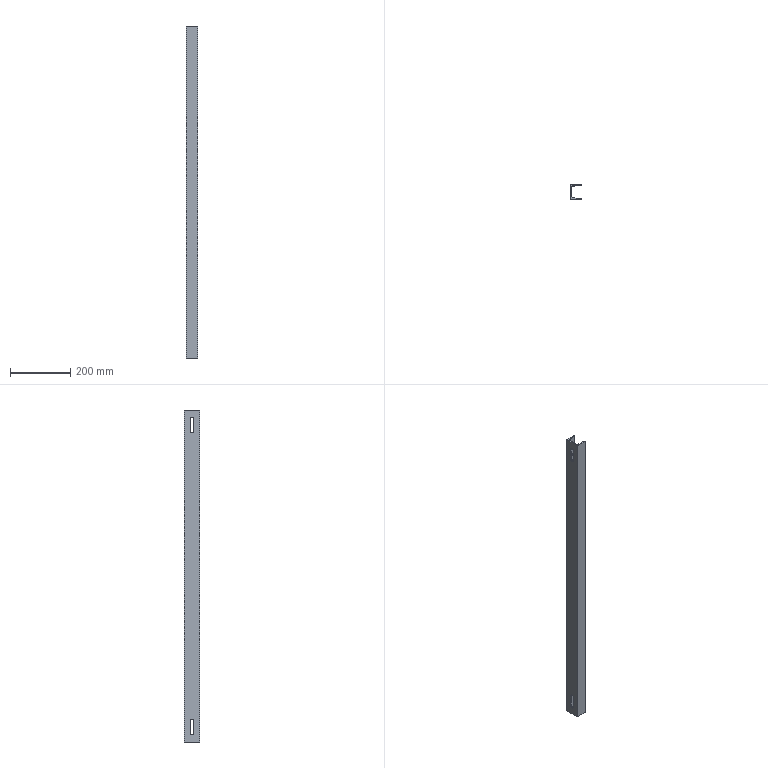Part | SolidWorks | features BaseBody 1 | 1 solid | 30 faces | box 37 x 50 x 1100 mm | volume 540936 mm3 | cylinder 18 | plane 12 | commonest cylinder face diameters 7 x6 12 x6 10.5 x4 14 x2
STEP:
#1=CARTESIAN_POINT('',(20.,21.002,446.5));
#2=VERTEX_POINT('',#1);
#3=CARTESIAN_POINT('',(20.,25.,446.5));
#4=VERTEX_POINT('',#3);
#5=CARTESIAN_POINT('',(20.,15.,446.5));
#6=DIRECTION('',(0.,1.,0.));
#7=VECTOR('',#6,1000.);
#8=LINE('',#5,#7);
#9=EDGE_CURVE('',#2,#4,#8,.T.);
#10=ORIENTED_EDGE('',*,*,#9,.F.);
#11=CARTESIAN_POINT('',(20.,21.002,453.5));
#12=VERTEX_POINT('',#11);
#13=CARTESIAN_POINT('',(20.,21.002,453.5));
#14=CARTESIAN_POINT('',(27.,21.259,453.5));
#15=CARTESIAN_POINT('',(27.,21.259,446.5));
#16=CARTESIAN_POINT('',(20.,21.002,446.5));
#17=(BOUNDED_CURVE()B_SPLINE_CURVE(3,(#13,#14,#15,#16),.UNSPECIFIED.,.F.,.F.)B_SPLINE_CURVE_WITH_KNOTS((4,4),(4.712,7.854),.UNSPECIFIED.)CURVE()GEOMETRIC_REPRESENTATION_ITEM()RATIONAL_B_SPLINE_CURVE((1.,0.3333,0.3333,1.))REPRESENTATION_ITEM(''));
#18=EDGE_CURVE('',#12,#2,#17,.T.);
#19=ORIENTED_EDGE('',*,*,#18,.F.);
#20=CARTESIAN_POINT('',(20.,25.,453.5));
#21=VERTEX_POINT('',#20);
#22=CARTESIAN_POINT('',(20.,15.,453.5));
#23=DIRECTION('',(0.,1.,0.));
#24=VECTOR('',#23,1000.);
#25=LINE('',#22,#24);
#26=EDGE_CURVE('',#12,#21,#25,.T.);
#27=ORIENTED_EDGE('',*,*,#26,.T.);
#28=CARTESIAN_POINT('',(20.,25.,450.));
#29=DIRECTION('',(0.,1.,0.));
#30=DIRECTION('',(0.,0.,1.));
#31=AXIS2_PLACEMENT_3D('',#28,#29,#30);
#32=CIRCLE('',#31,3.5);
#33=EDGE_CURVE('',#21,#4,#32,.T.);
#34=ORIENTED_EDGE('',*,*,#33,.T.);
#35=EDGE_LOOP('',(#10,#19,#27,#34));
#36=FACE_OUTER_BOUND('',#35,.T.);
#37=CARTESIAN_POINT('',(20.,15.,450.));
#38=DIRECTION('',(0.,1.,0.));
#39=DIRECTION('',(0.,0.,1.));
#40=AXIS2_PLACEMENT_3D('',#37,#38,#39);
#41=CYLINDRICAL_SURFACE('',#40,3.5);
#42=ADVANCED_FACE('',(#36),#41,.F.);
#43=CARTESIAN_POINT('',(20.,21.002,476.5));
#44=VERTEX_POINT('',#43);
#45=CARTESIAN_POINT('',(20.,25.,476.5));
#46=VERTEX_POINT('',#45);
#47=CARTESIAN_POINT('',(20.,15.,476.5));
#48=DIRECTION('',(0.,1.,0.));
#49=VECTOR('',#48,1000.);
#50=LINE('',#47,#49);
#51=EDGE_CURVE('',#44,#46,#50,.T.);
#52=ORIENTED_EDGE('',*,*,#51,.F.);
#53=CARTESIAN_POINT('',(20.,21.002,483.5));
#54=VERTEX_POINT('',#53);
#55=CARTESIAN_POINT('',(20.,21.002,483.5));
#56=CARTESIAN_POINT('',(27.,21.259,483.5));
#57=CARTESIAN_POINT('',(27.,21.259,476.5));
#58=CARTESIAN_POINT('',(20.,21.002,476.5));
#59=(BOUNDED_CURVE()B_SPLINE_CURVE(3,(#55,#56,#57,#58),.UNSPECIFIED.,.F.,.F.)B_SPLINE_CURVE_WITH_KNOTS((4,4),(4.712,7.854),.UNSPECIFIED.)CURVE()GEOMETRIC_REPRESENTATION_ITEM()RATIONAL_B_SPLINE_CURVE((1.,0.3333,0.3333,1.))REPRESENTATION_ITEM(''));
#60=EDGE_CURVE('',#54,#44,#59,.T.);
#61=ORIENTED_EDGE('',*,*,#60,.F.);
#62=CARTESIAN_POINT('',(20.,25.,483.5));
#63=VERTEX_POINT('',#62);
#64=CARTESIAN_POINT('',(20.,15.,483.5));
#65=DIRECTION('',(0.,1.,0.));
#66=VECTOR('',#65,1000.);
#67=LINE('',#64,#66);
#68=EDGE_CURVE('',#54,#63,#67,.T.);
#69=ORIENTED_EDGE('',*,*,#68,.T.);
#70=CARTESIAN_POINT('',(20.,25.,480.));
#71=DIRECTION('',(0.,1.,0.));
#72=DIRECTION('',(0.,0.,1.));
#73=AXIS2_PLACEMENT_3D('',#70,#71,#72);
#74=CIRCLE('',#73,3.5);
#75=EDGE_CURVE('',#63,#46,#74,.T.);
#76=ORIENTED_EDGE('',*,*,#75,.T.);
#77=EDGE_LOOP('',(#52,#61,#69,#76));
#78=FACE_OUTER_BOUND('',#77,.T.);
#79=CARTESIAN_POINT('',(20.,15.,480.));
#80=DIRECTION('',(0.,1.,0.));
#81=DIRECTION('',(0.,0.,1.));
#82=AXIS2_PLACEMENT_3D('',#79,#80,#81);
#83=CYLINDRICAL_SURFACE('',#82,3.5);
#84=ADVANCED_FACE('',(#78),#83,.F.);
#85=CARTESIAN_POINT('',(18.5,20.947,109.75));
#86=VERTEX_POINT('',#85);
#87=CARTESIAN_POINT('',(18.5,25.,109.75));
#88=VERTEX_POINT('',#87);
#89=CARTESIAN_POINT('',(18.5,-5.,109.75));
#90=DIRECTION('',(0.,1.,0.));
#91=VECTOR('',#90,1000.);
#92=LINE('',#89,#91);
#93=EDGE_CURVE('',#86,#88,#92,.T.);
#94=ORIENTED_EDGE('',*,*,#93,.F.);
#95=CARTESIAN_POINT('',(18.5,20.947,120.25));
#96=VERTEX_POINT('',#95);
#97=CARTESIAN_POINT('',(18.5,20.947,120.25));
#98=CARTESIAN_POINT('',(29.,21.333,120.25));
#99=CARTESIAN_POINT('',(29.,21.333,109.75));
#100=CARTESIAN_POINT('',(18.5,20.947,109.75));
#101=(BOUNDED_CURVE()B_SPLINE_CURVE(3,(#97,#98,#99,#100),.UNSPECIFIED.,.F.,.F.)B_SPLINE_CURVE_WITH_KNOTS((4,4),(4.712,7.854),.UNSPECIFIED.)CURVE()GEOMETRIC_REPRESENTATION_ITEM()RATIONAL_B_SPLINE_CURVE((1.,0.3333,0.3333,1.))REPRESENTATION_ITEM(''));
#102=EDGE_CURVE('',#96,#86,#101,.T.);
#103=ORIENTED_EDGE('',*,*,#102,.F.);
#104=CARTESIAN_POINT('',(18.5,25.,120.25));
#105=VERTEX_POINT('',#104);
#106=CARTESIAN_POINT('',(18.5,-5.,120.25));
#107=DIRECTION('',(0.,1.,0.));
#108=VECTOR('',#107,1000.);
#109=LINE('',#106,#108);
#110=EDGE_CURVE('',#96,#105,#109,.T.);
#111=ORIENTED_EDGE('',*,*,#110,.T.);
#112=CARTESIAN_POINT('',(18.5,25.,115.));
#113=DIRECTION('',(0.,1.,0.));
#114=DIRECTION('',(0.,0.,1.));
#115=AXIS2_PLACEMENT_3D('',#112,#113,#114);
#116=CIRCLE('',#115,5.25);
#117=EDGE_CURVE('',#105,#88,#116,.T.);
#118=ORIENTED_EDGE('',*,*,#117,.T.);
#119=EDGE_LOOP('',(#94,#103,#111,#118));
#120=FACE_OUTER_BOUND('',#119,.T.);
#121=CARTESIAN_POINT('',(18.5,-5.,115.));
#122=DIRECTION('',(0.,1.,0.));
#123=DIRECTION('',(0.,0.,1.));
#124=AXIS2_PLACEMENT_3D('',#121,#122,#123);
#125=CYLINDRICAL_SURFACE('',#124,5.25);
#126=ADVANCED_FACE('',(#120),#125,.F.);
#127=CARTESIAN_POINT('',(18.5,20.947,14.75));
#128=VERTEX_POINT('',#127);
#129=CARTESIAN_POINT('',(18.5,25.,14.75));
#130=VERTEX_POINT('',#129);
#131=CARTESIAN_POINT('',(18.5,-5.,14.75));
#132=DIRECTION('',(0.,1.,0.));
#133=VECTOR('',#132,1000.);
#134=LINE('',#131,#133);
#135=EDGE_CURVE('',#128,#130,#134,.T.);
#136=ORIENTED_EDGE('',*,*,#135,.F.);
#137=CARTESIAN_POINT('',(18.5,20.947,25.25));
#138=VERTEX_POINT('',#137);
#139=CARTESIAN_POINT('',(18.5,20.947,25.25));
#140=CARTESIAN_POINT('',(29.,21.333,25.25));
#141=CARTESIAN_POINT('',(29.,21.333,14.75));
#142=CARTESIAN_POINT('',(18.5,20.947,14.75));
#143=(BOUNDED_CURVE()B_SPLINE_CURVE(3,(#139,#140,#141,#142),.UNSPECIFIED.,.F.,.F.)B_SPLINE_CURVE_WITH_KNOTS((4,4),(4.712,7.854),.UNSPECIFIED.)CURVE()GEOMETRIC_REPRESENTATION_ITEM()RATIONAL_B_SPLINE_CURVE((1.,0.3333,0.3333,1.))REPRESENTATION_ITEM(''));
#144=EDGE_CURVE('',#138,#128,#143,.T.);
#145=ORIENTED_EDGE('',*,*,#144,.F.);
#146=CARTESIAN_POINT('',(18.5,25.,25.25));
#147=VERTEX_POINT('',#146);
#148=CARTESIAN_POINT('',(18.5,-5.,25.25));
#149=DIRECTION('',(0.,1.,0.));
#150=VECTOR('',#149,1000.);
#151=LINE('',#148,#150);
#152=EDGE_CURVE('',#138,#147,#151,.T.);
#153=ORIENTED_EDGE('',*,*,#152,.T.);
#154=CARTESIAN_POINT('',(18.5,25.,20.));
#155=DIRECTION('',(0.,1.,0.));
#156=DIRECTION('',(0.,0.,1.));
#157=AXIS2_PLACEMENT_3D('',#154,#155,#156);
#158=CIRCLE('',#157,5.25);
#159=EDGE_CURVE('',#147,#130,#158,.T.);
#160=ORIENTED_EDGE('',*,*,#159,.T.);
#161=EDGE_LOOP('',(#136,#145,#153,#160));
#162=FACE_OUTER_BOUND('',#161,.T.);
#163=CARTESIAN_POINT('',(18.5,-5.,20.));
#164=DIRECTION('',(0.,1.,0.));
#165=DIRECTION('',(0.,0.,1.));
#166=AXIS2_PLACEMENT_3D('',#163,#164,#165);
#167=CYLINDRICAL_SURFACE('',#166,5.25);
#168=ADVANCED_FACE('',(#162),#167,.F.);
#169=CARTESIAN_POINT('',(4.5,-6.,-520.));
#170=VERTEX_POINT('',#169);
#171=CARTESIAN_POINT('',(0.,-6.,-520.));
#172=VERTEX_POINT('',#171);
#173=CARTESIAN_POINT('',(10.,-6.,-520.));
#174=DIRECTION('',(-1.,0.,0.));
#175=VECTOR('',#174,1000.);
#176=LINE('',#173,#175);
#177=EDGE_CURVE('',#170,#172,#176,.T.);
#178=ORIENTED_EDGE('',*,*,#177,.T.);
#179=CARTESIAN_POINT('',(0.,-6.,-480.));
#180=VERTEX_POINT('',#179);
#181=CARTESIAN_POINT('',(0.,-6.,-520.));
#182=DIRECTION('',(0.,0.,1.));
#183=VECTOR('',#182,1000.);
#184=LINE('',#181,#183);
#185=EDGE_CURVE('',#172,#180,#184,.T.);
#186=ORIENTED_EDGE('',*,*,#185,.T.);
#187=CARTESIAN_POINT('',(4.5,-6.,-480.));
#188=VERTEX_POINT('',#187);
#189=CARTESIAN_POINT('',(10.,-6.,-480.));
#190=DIRECTION('',(-1.,0.,0.));
#191=VECTOR('',#190,1000.);
#192=LINE('',#189,#191);
#193=EDGE_CURVE('',#188,#180,#192,.T.);
#194=ORIENTED_EDGE('',*,*,#193,.F.);
#195=CARTESIAN_POINT('',(4.5,-6.,550.));
#196=DIRECTION('',(0.,0.,1.));
#197=VECTOR('',#196,1000.);
#198=LINE('',#195,#197);
#199=EDGE_CURVE('',#170,#188,#198,.T.);
#200=ORIENTED_EDGE('',*,*,#199,.F.);
#201=EDGE_LOOP('',(#178,#186,#194,#200));
#202=FACE_OUTER_BOUND('',#201,.T.);
#203=CARTESIAN_POINT('',(10.,-6.,-520.));
#204=DIRECTION('',(0.,-1.,0.));
#205=DIRECTION('',(0.,0.,-1.));
#206=AXIS2_PLACEMENT_3D('',#203,#204,#205);
#207=PLANE('',#206);
#208=ADVANCED_FACE('',(#202),#207,.F.);
#209=CARTESIAN_POINT('',(4.5,0.,-474.));
#210=VERTEX_POINT('',#209);
#211=CARTESIAN_POINT('',(0.,0.,-474.));
#212=VERTEX_POINT('',#211);
#213=CARTESIAN_POINT('',(10.,0.,-474.));
#214=DIRECTION('',(-1.,0.,0.));
#215=VECTOR('',#214,1000.);
#216=LINE('',#213,#215);
#217=EDGE_CURVE('',#210,#212,#216,.T.);
#218=ORIENTED_EDGE('',*,*,#217,.F.);
#219=CARTESIAN_POINT('',(4.5,0.,-480.));
#220=DIRECTION('',(-1.,0.,0.));
#221=DIRECTION('',(0.,0.,1.));
#222=AXIS2_PLACEMENT_3D('',#219,#220,#221);
#223=CIRCLE('',#222,6.);
#224=EDGE_CURVE('',#188,#210,#223,.T.);
#225=ORIENTED_EDGE('',*,*,#224,.F.);
#226=ORIENTED_EDGE('',*,*,#193,.T.);
#227=CARTESIAN_POINT('',(0.,0.,-480.));
#228=DIRECTION('',(-1.,0.,0.));
#229=DIRECTION('',(0.,0.,1.));
#230=AXIS2_PLACEMENT_3D('',#227,#228,#229);
#231=CIRCLE('',#230,6.);
#232=EDGE_CURVE('',#180,#212,#231,.T.);
#233=ORIENTED_EDGE('',*,*,#232,.T.);
#234=EDGE_LOOP('',(#218,#225,#226,#233));
#235=FACE_OUTER_BOUND('',#234,.T.);
#236=CARTESIAN_POINT('',(10.,0.,-480.));
#237=DIRECTION('',(-1.,0.,0.));
#238=DIRECTION('',(0.,0.,1.));
#239=AXIS2_PLACEMENT_3D('',#236,#237,#238);
#240=CYLINDRICAL_SURFACE('',#239,6.);
#241=ADVANCED_FACE('',(#235),#240,.F.);
#242=CARTESIAN_POINT('',(4.5,6.,-480.));
#243=VERTEX_POINT('',#242);
#244=CARTESIAN_POINT('',(0.,6.,-480.));
#245=VERTEX_POINT('',#244);
#246=CARTESIAN_POINT('',(10.,6.,-480.));
#247=DIRECTION('',(-1.,0.,0.));
#248=VECTOR('',#247,1000.);
#249=LINE('',#246,#248);
#250=EDGE_CURVE('',#243,#245,#249,.T.);
#251=ORIENTED_EDGE('',*,*,#250,.T.);
#252=CARTESIAN_POINT('',(0.,6.,-520.));
#253=VERTEX_POINT('',#252);
#254=CARTESIAN_POINT('',(0.,6.,-520.));
#255=DIRECTION('',(0.,0.,-1.));
#256=VECTOR('',#255,1000.);
#257=LINE('',#254,#256);
#258=EDGE_CURVE('',#245,#253,#257,.T.);
#259=ORIENTED_EDGE('',*,*,#258,.T.);
#260=CARTESIAN_POINT('',(4.5,6.,-520.));
#261=VERTEX_POINT('',#260);
#262=CARTESIAN_POINT('',(10.,6.,-520.));
#263=DIRECTION('',(-1.,0.,0.));
#264=VECTOR('',#263,1000.);
#265=LINE('',#262,#264);
#266=EDGE_CURVE('',#261,#253,#265,.T.);
#267=ORIENTED_EDGE('',*,*,#266,.F.);
#268=CARTESIAN_POINT('',(4.5,6.,550.));
#269=DIRECTION('',(0.,0.,-1.));
#270=VECTOR('',#269,1000.);
#271=LINE('',#268,#270);
#272=EDGE_CURVE('',#243,#261,#271,.T.);
#273=ORIENTED_EDGE('',*,*,#272,.F.);
#274=EDGE_LOOP('',(#251,#259,#267,#273));
#275=FACE_OUTER_BOUND('',#274,.T.);
#276=CARTESIAN_POINT('',(10.,6.,-520.));
#277=DIRECTION('',(0.,1.,0.));
#278=DIRECTION('',(1.,0.,0.));
#279=AXIS2_PLACEMENT_3D('',#276,#277,#278);
#280=PLANE('',#279);
#281=ADVANCED_FACE('',(#275),#280,.F.);
#282=ORIENTED_EDGE('',*,*,#266,.T.);
#283=CARTESIAN_POINT('',(0.,0.,-520.));
#284=DIRECTION('',(-1.,0.,0.));
#285=DIRECTION('',(0.,0.,1.));
#286=AXIS2_PLACEMENT_3D('',#283,#284,#285);
#287=CIRCLE('',#286,6.);
#288=EDGE_CURVE('',#253,#172,#287,.T.);
#289=ORIENTED_EDGE('',*,*,#288,.T.);
#290=ORIENTED_EDGE('',*,*,#177,.F.);
#291=CARTESIAN_POINT('',(4.5,0.,-520.));
#292=DIRECTION('',(-1.,0.,0.));
#293=DIRECTION('',(0.,0.,1.));
#294=AXIS2_PLACEMENT_3D('',#291,#292,#293);
#295=CIRCLE('',#294,6.);
#296=EDGE_CURVE('',#261,#170,#295,.T.);
#297=ORIENTED_EDGE('',*,*,#296,.F.);
#298=EDGE_LOOP('',(#282,#289,#290,#297));
#299=FACE_OUTER_BOUND('',#298,.T.);
#300=CARTESIAN_POINT('',(10.,0.,-520.));
#301=DIRECTION('',(-1.,0.,0.));
#302=DIRECTION('',(0.,0.,1.));
#303=AXIS2_PLACEMENT_3D('',#300,#301,#302);
#304=CYLINDRICAL_SURFACE('',#303,6.);
#305=ADVANCED_FACE('',(#299),#304,.F.);
#306=CARTESIAN_POINT('',(4.5,6.,520.));
#307=VERTEX_POINT('',#306);
#308=CARTESIAN_POINT('',(0.,6.,520.));
#309=VERTEX_POINT('',#308);
#310=CARTESIAN_POINT('',(10.,6.,520.));
#311=DIRECTION('',(-1.,0.,0.));
#312=VECTOR('',#311,1000.);
#313=LINE('',#310,#312);
#314=EDGE_CURVE('',#307,#309,#313,.T.);
#315=ORIENTED_EDGE('',*,*,#314,.T.);
#316=CARTESIAN_POINT('',(0.,6.,480.));
#317=VERTEX_POINT('',#316);
#318=CARTESIAN_POINT('',(0.,6.,520.));
#319=DIRECTION('',(0.,0.,-1.));
#320=VECTOR('',#319,1000.);
#321=LINE('',#318,#320);
#322=EDGE_CURVE('',#309,#317,#321,.T.);
#323=ORIENTED_EDGE('',*,*,#322,.T.);
#324=CARTESIAN_POINT('',(4.5,6.,480.));
#325=VERTEX_POINT('',#324);
#326=CARTESIAN_POINT('',(10.,6.,480.));
#327=DIRECTION('',(-1.,0.,0.));
#328=VECTOR('',#327,1000.);
#329=LINE('',#326,#328);
#330=EDGE_CURVE('',#325,#317,#329,.T.);
#331=ORIENTED_EDGE('',*,*,#330,.F.);
#332=CARTESIAN_POINT('',(4.5,6.,550.));
#333=DIRECTION('',(0.,0.,-1.));
#334=VECTOR('',#333,1000.);
#335=LINE('',#332,#334);
#336=EDGE_CURVE('',#307,#325,#335,.T.);
#337=ORIENTED_EDGE('',*,*,#336,.F.);
#338=EDGE_LOOP('',(#315,#323,#331,#337));
#339=FACE_OUTER_BOUND('',#338,.T.);
#340=CARTESIAN_POINT('',(10.,6.,520.));
#341=DIRECTION('',(0.,1.,0.));
#342=DIRECTION('',(1.,0.,0.));
#343=AXIS2_PLACEMENT_3D('',#340,#341,#342);
#344=PLANE('',#343);
#345=ADVANCED_FACE('',(#339),#344,.F.);
#346=ORIENTED_EDGE('',*,*,#330,.T.);
#347=CARTESIAN_POINT('',(0.,-6.,480.));
#348=VERTEX_POINT('',#347);
#349=CARTESIAN_POINT('',(0.,0.,480.));
#350=DIRECTION('',(-1.,0.,0.));
#351=DIRECTION('',(0.,0.,-1.));
#352=AXIS2_PLACEMENT_3D('',#349,#350,#351);
#353=CIRCLE('',#352,6.);
#354=EDGE_CURVE('',#317,#348,#353,.T.);
#355=ORIENTED_EDGE('',*,*,#354,.T.);
#356=CARTESIAN_POINT('',(4.5,-6.,480.));
#357=VERTEX_POINT('',#356);
#358=CARTESIAN_POINT('',(10.,-6.,480.));
#359=DIRECTION('',(-1.,0.,0.));
#360=VECTOR('',#359,1000.);
#361=LINE('',#358,#360);
#362=EDGE_CURVE('',#357,#348,#361,.T.);
#363=ORIENTED_EDGE('',*,*,#362,.F.);
#364=CARTESIAN_POINT('',(4.5,0.,480.));
#365=DIRECTION('',(-1.,0.,0.));
#366=DIRECTION('',(0.,0.,1.));
#367=AXIS2_PLACEMENT_3D('',#364,#365,#366);
#368=CIRCLE('',#367,6.);
#369=EDGE_CURVE('',#325,#357,#368,.T.);
#370=ORIENTED_EDGE('',*,*,#369,.F.);
#371=EDGE_LOOP('',(#346,#355,#363,#370));
#372=FACE_OUTER_BOUND('',#371,.T.);
#373=CARTESIAN_POINT('',(10.,0.,480.));
#374=DIRECTION('',(-1.,0.,0.));
#375=DIRECTION('',(0.,0.,1.));
#376=AXIS2_PLACEMENT_3D('',#373,#374,#375);
#377=CYLINDRICAL_SURFACE('',#376,6.);
#378=ADVANCED_FACE('',(#372),#377,.F.);
#379=ORIENTED_EDGE('',*,*,#362,.T.);
#380=CARTESIAN_POINT('',(0.,-6.,520.));
#381=VERTEX_POINT('',#380);
#382=CARTESIAN_POINT('',(0.,-6.,520.));
#383=DIRECTION('',(0.,0.,1.));
#384=VECTOR('',#383,1000.);
#385=LINE('',#382,#384);
#386=EDGE_CURVE('',#348,#381,#385,.T.);
#387=ORIENTED_EDGE('',*,*,#386,.T.);
#388=CARTESIAN_POINT('',(4.5,-6.,520.));
#389=VERTEX_POINT('',#388);
#390=CARTESIAN_POINT('',(10.,-6.,520.));
#391=DIRECTION('',(-1.,0.,0.));
#392=VECTOR('',#391,1000.);
#393=LINE('',#390,#392);
#394=EDGE_CURVE('',#389,#381,#393,.T.);
#395=ORIENTED_EDGE('',*,*,#394,.F.);
#396=CARTESIAN_POINT('',(4.5,-6.,550.));
#397=DIRECTION('',(0.,0.,1.));
#398=VECTOR('',#397,1000.);
#399=LINE('',#396,#398);
#400=EDGE_CURVE('',#357,#389,#399,.T.);
#401=ORIENTED_EDGE('',*,*,#400,.F.);
#402=EDGE_LOOP('',(#379,#387,#395,#401));
#403=FACE_OUTER_BOUND('',#402,.T.);
#404=CARTESIAN_POINT('',(10.,-6.,520.));
#405=DIRECTION('',(0.,-1.,0.));
#406=DIRECTION('',(0.,0.,-1.));
#407=AXIS2_PLACEMENT_3D('',#404,#405,#406);
#408=PLANE('',#407);
#409=ADVANCED_FACE('',(#403),#408,.F.);
#410=CARTESIAN_POINT('',(4.5,0.,526.));
#411=VERTEX_POINT('',#410);
#412=CARTESIAN_POINT('',(0.,0.,526.));
#413=VERTEX_POINT('',#412);
#414=CARTESIAN_POINT('',(10.,0.,526.));
#415=DIRECTION('',(-1.,0.,0.));
#416=VECTOR('',#415,1000.);
#417=LINE('',#414,#416);
#418=EDGE_CURVE('',#411,#413,#417,.T.);
#419=ORIENTED_EDGE('',*,*,#418,.F.);
#420=CARTESIAN_POINT('',(4.5,0.,520.));
#421=DIRECTION('',(-1.,0.,0.));
#422=DIRECTION('',(0.,0.,1.));
#423=AXIS2_PLACEMENT_3D('',#420,#421,#422);
#424=CIRCLE('',#423,6.);
#425=EDGE_CURVE('',#389,#411,#424,.T.);
#426=ORIENTED_EDGE('',*,*,#425,.F.);
#427=ORIENTED_EDGE('',*,*,#394,.T.);
#428=CARTESIAN_POINT('',(0.,0.,520.));
#429=DIRECTION('',(-1.,0.,0.));
#430=DIRECTION('',(0.,0.,-1.));
#431=AXIS2_PLACEMENT_3D('',#428,#429,#430);
#432=CIRCLE('',#431,6.);
#433=EDGE_CURVE('',#381,#413,#432,.T.);
#434=ORIENTED_EDGE('',*,*,#433,.T.);
#435=EDGE_LOOP('',(#419,#426,#427,#434));
#436=FACE_OUTER_BOUND('',#435,.T.);
#437=CARTESIAN_POINT('',(10.,0.,520.));
#438=DIRECTION('',(-1.,0.,0.));
#439=DIRECTION('',(0.,0.,1.));
#440=AXIS2_PLACEMENT_3D('',#437,#438,#439);
#441=CYLINDRICAL_SURFACE('',#440,6.);
#442=ADVANCED_FACE('',(#436),#441,.F.);
#443=CARTESIAN_POINT('',(0.,-25.,-550.));
#444=VERTEX_POINT('',#443);
#445=CARTESIAN_POINT('',(37.,-25.,-550.));
#446=VERTEX_POINT('',#445);
#447=CARTESIAN_POINT('',(0.,-25.,-550.));
#448=DIRECTION('',(1.,0.,0.));
#449=VECTOR('',#448,1000.);
#450=LINE('',#447,#449);
#451=EDGE_CURVE('',#444,#446,#450,.T.);
#452=ORIENTED_EDGE('',*,*,#451,.F.);
#453=CARTESIAN_POINT('',(0.,25.,-550.));
#454=VERTEX_POINT('',#453);
#455=CARTESIAN_POINT('',(0.,-25.,-550.));
#456=DIRECTION('',(0.,-1.,0.));
#457=VECTOR('',#456,1000.);
#458=LINE('',#455,#457);
#459=EDGE_CURVE('',#454,#444,#458,.T.);
#460=ORIENTED_EDGE('',*,*,#459,.F.);
#461=CARTESIAN_POINT('',(37.,25.,-550.));
#462=VERTEX_POINT('',#461);
#463=CARTESIAN_POINT('',(0.,25.,-550.));
#464=DIRECTION('',(-1.,0.,0.));
#465=VECTOR('',#464,1000.);
#466=LINE('',#463,#465);
#467=EDGE_CURVE('',#462,#454,#466,.T.);
#468=ORIENTED_EDGE('',*,*,#467,.F.);
#469=CARTESIAN_POINT('',(33.628,21.502,-550.));
#470=VERTEX_POINT('',#469);
#471=CARTESIAN_POINT('',(33.5,25.,-550.));
#472=DIRECTION('',(0.,0.,1.));
#473=DIRECTION('',(1.,0.,0.));
#474=AXIS2_PLACEMENT_3D('',#471,#472,#473);
#475=CIRCLE('',#474,3.5);
#476=EDGE_CURVE('',#470,#462,#475,.T.);
#477=ORIENTED_EDGE('',*,*,#476,.F.);
#478=CARTESIAN_POINT('',(11.243,20.681,-550.));
#479=VERTEX_POINT('',#478);
#480=CARTESIAN_POINT('',(11.243,20.681,-550.));
#481=DIRECTION('',(0.9993,0.03666,0.));
#482=VECTOR('',#481,1000.);
#483=LINE('',#480,#482);
#484=EDGE_CURVE('',#479,#470,#483,.T.);
#485=ORIENTED_EDGE('',*,*,#484,.F.);
#486=CARTESIAN_POINT('',(4.5,13.686,-550.));
#487=VERTEX_POINT('',#486);
#488=CARTESIAN_POINT('',(11.5,13.686,-550.));
#489=DIRECTION('',(0.,0.,-1.));
#490=DIRECTION('',(1.,0.,0.));
#491=AXIS2_PLACEMENT_3D('',#488,#489,#490);
#492=CIRCLE('',#491,7.);
#493=EDGE_CURVE('',#487,#479,#492,.T.);
#494=ORIENTED_EDGE('',*,*,#493,.F.);
#495=CARTESIAN_POINT('',(4.5,-13.686,-550.));
#496=VERTEX_POINT('',#495);
#497=CARTESIAN_POINT('',(4.5,-13.686,-550.));
#498=DIRECTION('',(0.,1.,0.));
#499=VECTOR('',#498,1000.);
#500=LINE('',#497,#499);
#501=EDGE_CURVE('',#496,#487,#500,.T.);
#502=ORIENTED_EDGE('',*,*,#501,.F.);
#503=CARTESIAN_POINT('',(11.243,-20.681,-550.));
#504=VERTEX_POINT('',#503);
#505=CARTESIAN_POINT('',(11.5,-13.686,-550.));
#506=DIRECTION('',(0.,0.,-1.));
#507=DIRECTION('',(1.,0.,0.));
#508=AXIS2_PLACEMENT_3D('',#505,#506,#507);
#509=CIRCLE('',#508,7.);
#510=EDGE_CURVE('',#504,#496,#509,.T.);
#511=ORIENTED_EDGE('',*,*,#510,.F.);
#512=CARTESIAN_POINT('',(33.628,-21.502,-550.));
#513=VERTEX_POINT('',#512);
#514=CARTESIAN_POINT('',(11.243,-20.681,-550.));
#515=DIRECTION('',(-0.9993,0.03666,0.));
#516=VECTOR('',#515,1000.);
#517=LINE('',#514,#516);
#518=EDGE_CURVE('',#513,#504,#517,.T.);
#519=ORIENTED_EDGE('',*,*,#518,.F.);
#520=CARTESIAN_POINT('',(33.5,-25.,-550.));
#521=DIRECTION('',(0.,0.,1.));
#522=DIRECTION('',(-1.,0.,0.));
#523=AXIS2_PLACEMENT_3D('',#520,#521,#522);
#524=CIRCLE('',#523,3.5);
#525=EDGE_CURVE('',#446,#513,#524,.T.);
#526=ORIENTED_EDGE('',*,*,#525,.F.);
#527=EDGE_LOOP('',(#452,#460,#468,#477,#485,#494,#502,#511,#519,#526));
#528=FACE_OUTER_BOUND('',#527,.T.);
#529=CARTESIAN_POINT('',(33.5,-25.,-550.));
#530=DIRECTION('',(0.,0.,-1.));
#531=DIRECTION('',(0.,-1.,0.));
#532=AXIS2_PLACEMENT_3D('',#529,#530,#531);
#533=PLANE('',#532);
#534=ADVANCED_FACE('',(#528),#533,.T.);
#535=CARTESIAN_POINT('',(0.,-25.,550.));
#536=VERTEX_POINT('',#535);
#537=CARTESIAN_POINT('',(37.,-25.,550.));
#538=VERTEX_POINT('',#537);
#539=CARTESIAN_POINT('',(0.,-25.,550.));
#540=DIRECTION('',(1.,0.,0.));
#541=VECTOR('',#540,1000.);
#542=LINE('',#539,#541);
#543=EDGE_CURVE('',#536,#538,#542,.T.);
#544=ORIENTED_EDGE('',*,*,#543,.T.);
#545=CARTESIAN_POINT('',(33.628,-21.502,550.));
#546=VERTEX_POINT('',#545);
#547=CARTESIAN_POINT('',(33.5,-25.,550.));
#548=DIRECTION('',(0.,0.,1.));
#549=DIRECTION('',(-1.,0.,0.));
#550=AXIS2_PLACEMENT_3D('',#547,#548,#549);
#551=CIRCLE('',#550,3.5);
#552=EDGE_CURVE('',#538,#546,#551,.T.);
#553=ORIENTED_EDGE('',*,*,#552,.T.);
#554=CARTESIAN_POINT('',(11.243,-20.681,550.));
#555=VERTEX_POINT('',#554);
#556=CARTESIAN_POINT('',(11.243,-20.681,550.));
#557=DIRECTION('',(-0.9993,0.03666,0.));
#558=VECTOR('',#557,1000.);
#559=LINE('',#556,#558);
#560=EDGE_CURVE('',#546,#555,#559,.T.);
#561=ORIENTED_EDGE('',*,*,#560,.T.);
#562=CARTESIAN_POINT('',(4.5,-13.686,550.));
#563=VERTEX_POINT('',#562);
#564=CARTESIAN_POINT('',(11.5,-13.686,550.));
#565=DIRECTION('',(0.,0.,-1.));
#566=DIRECTION('',(1.,0.,0.));
#567=AXIS2_PLACEMENT_3D('',#564,#565,#566);
#568=CIRCLE('',#567,7.);
#569=EDGE_CURVE('',#555,#563,#568,.T.);
#570=ORIENTED_EDGE('',*,*,#569,.T.);
#571=CARTESIAN_POINT('',(4.5,13.686,550.));
#572=VERTEX_POINT('',#571);
#573=CARTESIAN_POINT('',(4.5,-13.686,550.));
#574=DIRECTION('',(0.,1.,0.));
#575=VECTOR('',#574,1000.);
#576=LINE('',#573,#575);
#577=EDGE_CURVE('',#563,#572,#576,.T.);
#578=ORIENTED_EDGE('',*,*,#577,.T.);
#579=CARTESIAN_POINT('',(11.243,20.681,550.));
#580=VERTEX_POINT('',#579);
#581=CARTESIAN_POINT('',(11.5,13.686,550.));
#582=DIRECTION('',(0.,0.,-1.));
#583=DIRECTION('',(1.,0.,0.));
#584=AXIS2_PLACEMENT_3D('',#581,#582,#583);
#585=CIRCLE('',#584,7.);
#586=EDGE_CURVE('',#572,#580,#585,.T.);
#587=ORIENTED_EDGE('',*,*,#586,.T.);
#588=CARTESIAN_POINT('',(33.628,21.502,550.));
#589=VERTEX_POINT('',#588);
#590=CARTESIAN_POINT('',(11.243,20.681,550.));
#591=DIRECTION('',(0.9993,0.03666,0.));
#592=VECTOR('',#591,1000.);
#593=LINE('',#590,#592);
#594=EDGE_CURVE('',#580,#589,#593,.T.);
#595=ORIENTED_EDGE('',*,*,#594,.T.);
#596=CARTESIAN_POINT('',(37.,25.,550.));
#597=VERTEX_POINT('',#596);
#598=CARTESIAN_POINT('',(33.5,25.,550.));
#599=DIRECTION('',(0.,0.,1.));
#600=DIRECTION('',(1.,0.,0.));
#601=AXIS2_PLACEMENT_3D('',#598,#599,#600);
#602=CIRCLE('',#601,3.5);
#603=EDGE_CURVE('',#589,#597,#602,.T.);
#604=ORIENTED_EDGE('',*,*,#603,.T.);
#605=CARTESIAN_POINT('',(0.,25.,550.));
#606=VERTEX_POINT('',#605);
#607=CARTESIAN_POINT('',(0.,25.,550.));
#608=DIRECTION('',(-1.,0.,0.));
#609=VECTOR('',#608,1000.);
#610=LINE('',#607,#609);
#611=EDGE_CURVE('',#597,#606,#610,.T.);
#612=ORIENTED_EDGE('',*,*,#611,.T.);
#613=CARTESIAN_POINT('',(0.,-25.,550.));
#614=DIRECTION('',(0.,-1.,0.));
#615=VECTOR('',#614,1000.);
#616=LINE('',#613,#615);
#617=EDGE_CURVE('',#606,#536,#616,.T.);
#618=ORIENTED_EDGE('',*,*,#617,.T.);
#619=EDGE_LOOP('',(#544,#553,#561,#570,#578,#587,#595,#604,#612,#618));
#620=FACE_OUTER_BOUND('',#619,.T.);
#621=CARTESIAN_POINT('',(33.5,-25.,550.));
#622=DIRECTION('',(0.,0.,-1.));
#623=DIRECTION('',(0.,-1.,0.));
#624=AXIS2_PLACEMENT_3D('',#621,#622,#623);
#625=PLANE('',#624);
#626=ADVANCED_FACE('',(#620),#625,.F.);
#627=ORIENTED_EDGE('',*,*,#322,.F.);
#628=CARTESIAN_POINT('',(0.,0.,520.));
#629=DIRECTION('',(-1.,0.,0.));
#630=DIRECTION('',(0.,0.,-1.));
#631=AXIS2_PLACEMENT_3D('',#628,#629,#630);
#632=CIRCLE('',#631,6.);
#633=EDGE_CURVE('',#413,#309,#632,.T.);
#634=ORIENTED_EDGE('',*,*,#633,.F.);
#635=ORIENTED_EDGE('',*,*,#433,.F.);
#636=ORIENTED_EDGE('',*,*,#386,.F.);
#637=ORIENTED_EDGE('',*,*,#354,.F.);
#638=EDGE_LOOP('',(#627,#634,#635,#636,#637));
#639=FACE_BOUND('',#638,.T.);
#640=ORIENTED_EDGE('',*,*,#185,.F.);
#641=ORIENTED_EDGE('',*,*,#288,.F.);
#642=ORIENTED_EDGE('',*,*,#258,.F.);
#643=CARTESIAN_POINT('',(0.,0.,-480.));
#644=DIRECTION('',(-1.,0.,0.));
#645=DIRECTION('',(0.,0.,1.));
#646=AXIS2_PLACEMENT_3D('',#643,#644,#645);
#647=CIRCLE('',#646,6.);
#648=EDGE_CURVE('',#212,#245,#647,.T.);
#649=ORIENTED_EDGE('',*,*,#648,.F.);
#650=ORIENTED_EDGE('',*,*,#232,.F.);
#651=EDGE_LOOP('',(#640,#641,#642,#649,#650));
#652=FACE_BOUND('',#651,.T.);
#653=ORIENTED_EDGE('',*,*,#459,.T.);
#654=CARTESIAN_POINT('',(0.,-25.,550.));
#655=DIRECTION('',(0.,0.,-1.));
#656=VECTOR('',#655,1000.);
#657=LINE('',#654,#656);
#658=EDGE_CURVE('',#536,#444,#657,.T.);
#659=ORIENTED_EDGE('',*,*,#658,.F.);
#660=ORIENTED_EDGE('',*,*,#617,.F.);
#661=CARTESIAN_POINT('',(0.,25.,550.));
#662=DIRECTION('',(0.,0.,-1.));
#663=VECTOR('',#662,1000.);
#664=LINE('',#661,#663);
#665=EDGE_CURVE('',#606,#454,#664,.T.);
#666=ORIENTED_EDGE('',*,*,#665,.T.);
#667=EDGE_LOOP('',(#653,#659,#660,#666));
#668=FACE_OUTER_BOUND('',#667,.T.);
#669=CARTESIAN_POINT('',(0.,-25.,550.));
#670=DIRECTION('',(1.,0.,0.));
#671=DIRECTION('',(0.,1.,0.));
#672=AXIS2_PLACEMENT_3D('',#669,#670,#671);
#673=PLANE('',#672);
#674=ADVANCED_FACE('',(#639,#652,#668),#673,.F.);
#675=ORIENTED_EDGE('',*,*,#159,.F.);
#676=CARTESIAN_POINT('',(18.5,25.,20.));
#677=DIRECTION('',(0.,1.,0.));
#678=DIRECTION('',(0.,0.,1.));
#679=AXIS2_PLACEMENT_3D('',#676,#677,#678);
#680=CIRCLE('',#679,5.25);
#681=EDGE_CURVE('',#130,#147,#680,.T.);
#682=ORIENTED_EDGE('',*,*,#681,.F.);
#683=EDGE_LOOP('',(#675,#682));
#684=FACE_BOUND('',#683,.T.);
#685=ORIENTED_EDGE('',*,*,#117,.F.);
#686=CARTESIAN_POINT('',(18.5,25.,115.));
#687=DIRECTION('',(0.,1.,0.));
#688=DIRECTION('',(0.,0.,1.));
#689=AXIS2_PLACEMENT_3D('',#686,#687,#688);
#690=CIRCLE('',#689,5.25);
#691=EDGE_CURVE('',#88,#105,#690,.T.);
#692=ORIENTED_EDGE('',*,*,#691,.F.);
#693=EDGE_LOOP('',(#685,#692));
#694=FACE_BOUND('',#693,.T.);
#695=ORIENTED_EDGE('',*,*,#75,.F.);
#696=CARTESIAN_POINT('',(20.,25.,480.));
#697=DIRECTION('',(0.,1.,0.));
#698=DIRECTION('',(0.,0.,1.));
#699=AXIS2_PLACEMENT_3D('',#696,#697,#698);
#700=CIRCLE('',#699,3.5);
#701=EDGE_CURVE('',#46,#63,#700,.T.);
#702=ORIENTED_EDGE('',*,*,#701,.F.);
#703=EDGE_LOOP('',(#695,#702));
#704=FACE_BOUND('',#703,.T.);
#705=ORIENTED_EDGE('',*,*,#33,.F.);
#706=CARTESIAN_POINT('',(20.,25.,450.));
#707=DIRECTION('',(0.,1.,0.));
#708=DIRECTION('',(0.,0.,1.));
#709=AXIS2_PLACEMENT_3D('',#706,#707,#708);
#710=CIRCLE('',#709,3.5);
#711=EDGE_CURVE('',#4,#21,#710,.T.);
#712=ORIENTED_EDGE('',*,*,#711,.F.);
#713=EDGE_LOOP('',(#705,#712));
#714=FACE_BOUND('',#713,.T.);
#715=ORIENTED_EDGE('',*,*,#467,.T.);
#716=ORIENTED_EDGE('',*,*,#665,.F.);
#717=ORIENTED_EDGE('',*,*,#611,.F.);
#718=CARTESIAN_POINT('',(37.,25.,550.));
#719=DIRECTION('',(0.,0.,-1.));
#720=VECTOR('',#719,1000.);
#721=LINE('',#718,#720);
#722=EDGE_CURVE('',#597,#462,#721,.T.);
#723=ORIENTED_EDGE('',*,*,#722,.T.);
#724=EDGE_LOOP('',(#715,#716,#717,#723));
#725=FACE_OUTER_BOUND('',#724,.T.);
#726=CARTESIAN_POINT('',(0.,25.,550.));
#727=DIRECTION('',(0.,-1.,0.));
#728=DIRECTION('',(0.,0.,-1.));
#729=AXIS2_PLACEMENT_3D('',#726,#727,#728);
#730=PLANE('',#729);
#731=ADVANCED_FACE('',(#684,#694,#704,#714,#725),#730,.F.);
#732=ORIENTED_EDGE('',*,*,#476,.T.);
#733=ORIENTED_EDGE('',*,*,#722,.F.);
#734=ORIENTED_EDGE('',*,*,#603,.F.);
#735=CARTESIAN_POINT('',(33.628,21.502,550.));
#736=DIRECTION('',(0.,0.,-1.));
#737=VECTOR('',#736,1000.);
#738=LINE('',#735,#737);
#739=EDGE_CURVE('',#589,#470,#738,.T.);
#740=ORIENTED_EDGE('',*,*,#739,.T.);
#741=EDGE_LOOP('',(#732,#733,#734,#740));
#742=FACE_OUTER_BOUND('',#741,.T.);
#743=CARTESIAN_POINT('',(33.5,25.,550.));
#744=DIRECTION('',(0.,0.,-1.));
#745=DIRECTION('',(-1.,0.,0.));
#746=AXIS2_PLACEMENT_3D('',#743,#744,#745);
#747=CYLINDRICAL_SURFACE('',#746,3.5);
#748=ADVANCED_FACE('',(#742),#747,.T.);
#749=ORIENTED_EDGE('',*,*,#144,.T.);
#750=CARTESIAN_POINT('',(18.5,20.947,14.75));
#751=CARTESIAN_POINT('',(8.,20.562,14.75));
#752=CARTESIAN_POINT('',(8.,20.562,25.25));
#753=CARTESIAN_POINT('',(18.5,20.947,25.25));
#754=(BOUNDED_CURVE()B_SPLINE_CURVE(3,(#750,#751,#752,#753),.UNSPECIFIED.,.F.,.T.)B_SPLINE_CURVE_WITH_KNOTS((4,4),(1.571,4.712),.UNSPECIFIED.)CURVE()GEOMETRIC_REPRESENTATION_ITEM()RATIONAL_B_SPLINE_CURVE((1.,0.3333,0.3333,1.))REPRESENTATION_ITEM(''));
#755=EDGE_CURVE('',#128,#138,#754,.T.);
#756=ORIENTED_EDGE('',*,*,#755,.T.);
#757=EDGE_LOOP('',(#749,#756));
#758=FACE_BOUND('',#757,.T.);
#759=ORIENTED_EDGE('',*,*,#102,.T.);
#760=CARTESIAN_POINT('',(18.5,20.947,109.75));
#761=CARTESIAN_POINT('',(8.,20.562,109.75));
#762=CARTESIAN_POINT('',(8.,20.562,120.25));
#763=CARTESIAN_POINT('',(18.5,20.947,120.25));
#764=(BOUNDED_CURVE()B_SPLINE_CURVE(3,(#760,#761,#762,#763),.UNSPECIFIED.,.F.,.F.)B_SPLINE_CURVE_WITH_KNOTS((4,4),(1.571,4.712),.UNSPECIFIED.)CURVE()GEOMETRIC_REPRESENTATION_ITEM()RATIONAL_B_SPLINE_CURVE((1.,0.3333,0.3333,1.))REPRESENTATION_ITEM(''));
#765=EDGE_CURVE('',#86,#96,#764,.T.);
#766=ORIENTED_EDGE('',*,*,#765,.T.);
#767=EDGE_LOOP('',(#759,#766));
#768=FACE_BOUND('',#767,.T.);
#769=ORIENTED_EDGE('',*,*,#60,.T.);
#770=CARTESIAN_POINT('',(20.,21.002,476.5));
#771=CARTESIAN_POINT('',(13.,20.746,476.5));
#772=CARTESIAN_POINT('',(13.,20.746,483.5));
#773=CARTESIAN_POINT('',(20.,21.002,483.5));
#774=(BOUNDED_CURVE()B_SPLINE_CURVE(3,(#770,#771,#772,#773),.UNSPECIFIED.,.F.,.F.)B_SPLINE_CURVE_WITH_KNOTS((4,4),(1.571,4.712),.UNSPECIFIED.)CURVE()GEOMETRIC_REPRESENTATION_ITEM()RATIONAL_B_SPLINE_CURVE((1.,0.3333,0.3333,1.))REPRESENTATION_ITEM(''));
#775=EDGE_CURVE('',#44,#54,#774,.T.);
#776=ORIENTED_EDGE('',*,*,#775,.T.);
#777=EDGE_LOOP('',(#769,#776));
#778=FACE_BOUND('',#777,.T.);
#779=ORIENTED_EDGE('',*,*,#18,.T.);
#780=CARTESIAN_POINT('',(20.,21.002,446.5));
#781=CARTESIAN_POINT('',(13.,20.746,446.5));
#782=CARTESIAN_POINT('',(13.,20.746,453.5));
#783=CARTESIAN_POINT('',(20.,21.002,453.5));
#784=(BOUNDED_CURVE()B_SPLINE_CURVE(3,(#780,#781,#782,#783),.UNSPECIFIED.,.F.,.F.)B_SPLINE_CURVE_WITH_KNOTS((4,4),(1.571,4.712),.UNSPECIFIED.)CURVE()GEOMETRIC_REPRESENTATION_ITEM()RATIONAL_B_SPLINE_CURVE((1.,0.3333,0.3333,1.))REPRESENTATION_ITEM(''));
#785=EDGE_CURVE('',#2,#12,#784,.T.);
#786=ORIENTED_EDGE('',*,*,#785,.T.);
#787=EDGE_LOOP('',(#779,#786));
#788=FACE_BOUND('',#787,.T.);
#789=ORIENTED_EDGE('',*,*,#484,.T.);
#790=ORIENTED_EDGE('',*,*,#739,.F.);
#791=ORIENTED_EDGE('',*,*,#594,.F.);
#792=CARTESIAN_POINT('',(11.243,20.681,550.));
#793=DIRECTION('',(0.,0.,-1.));
#794=VECTOR('',#793,1000.);
#795=LINE('',#792,#794);
#796=EDGE_CURVE('',#580,#479,#795,.T.);
#797=ORIENTED_EDGE('',*,*,#796,.T.);
#798=EDGE_LOOP('',(#789,#790,#791,#797));
#799=FACE_OUTER_BOUND('',#798,.T.);
#800=CARTESIAN_POINT('',(11.243,20.681,550.));
#801=DIRECTION('',(-0.03666,0.9993,0.));
#802=DIRECTION('',(0.,0.,1.));
#803=AXIS2_PLACEMENT_3D('',#800,#801,#802);
#804=PLANE('',#803);
#805=ADVANCED_FACE('',(#758,#768,#778,#788,#799),#804,.F.);
#806=ORIENTED_EDGE('',*,*,#493,.T.);
#807=ORIENTED_EDGE('',*,*,#796,.F.);
#808=ORIENTED_EDGE('',*,*,#586,.F.);
#809=CARTESIAN_POINT('',(4.5,13.686,550.));
#810=DIRECTION('',(0.,0.,-1.));
#811=VECTOR('',#810,1000.);
#812=LINE('',#809,#811);
#813=EDGE_CURVE('',#572,#487,#812,.T.);
#814=ORIENTED_EDGE('',*,*,#813,.T.);
#815=EDGE_LOOP('',(#806,#807,#808,#814));
#816=FACE_OUTER_BOUND('',#815,.T.);
#817=CARTESIAN_POINT('',(11.5,13.686,550.));
#818=DIRECTION('',(0.,0.,-1.));
#819=DIRECTION('',(-1.,0.,0.));
#820=AXIS2_PLACEMENT_3D('',#817,#818,#819);
#821=CYLINDRICAL_SURFACE('',#820,7.);
#822=ADVANCED_FACE('',(#816),#821,.F.);
#823=ORIENTED_EDGE('',*,*,#400,.T.);
#824=ORIENTED_EDGE('',*,*,#425,.T.);
#825=CARTESIAN_POINT('',(4.5,0.,520.));
#826=DIRECTION('',(-1.,0.,0.));
#827=DIRECTION('',(0.,0.,1.));
#828=AXIS2_PLACEMENT_3D('',#825,#826,#827);
#829=CIRCLE('',#828,6.);
#830=EDGE_CURVE('',#411,#307,#829,.T.);
#831=ORIENTED_EDGE('',*,*,#830,.T.);
#832=ORIENTED_EDGE('',*,*,#336,.T.);
#833=ORIENTED_EDGE('',*,*,#369,.T.);
#834=EDGE_LOOP('',(#823,#824,#831,#832,#833));
#835=FACE_BOUND('',#834,.T.);
#836=ORIENTED_EDGE('',*,*,#272,.T.);
#837=ORIENTED_EDGE('',*,*,#296,.T.);
#838=ORIENTED_EDGE('',*,*,#199,.T.);
#839=ORIENTED_EDGE('',*,*,#224,.T.);
#840=CARTESIAN_POINT('',(4.5,0.,-480.));
#841=DIRECTION('',(-1.,0.,0.));
#842=DIRECTION('',(0.,0.,1.));
#843=AXIS2_PLACEMENT_3D('',#840,#841,#842);
#844=CIRCLE('',#843,6.);
#845=EDGE_CURVE('',#210,#243,#844,.T.);
#846=ORIENTED_EDGE('',*,*,#845,.T.);
#847=EDGE_LOOP('',(#836,#837,#838,#839,#846));
#848=FACE_BOUND('',#847,.T.);
#849=ORIENTED_EDGE('',*,*,#501,.T.);
#850=ORIENTED_EDGE('',*,*,#813,.F.);
#851=ORIENTED_EDGE('',*,*,#577,.F.);
#852=CARTESIAN_POINT('',(4.5,-13.686,550.));
#853=DIRECTION('',(0.,0.,-1.));
#854=VECTOR('',#853,1000.);
#855=LINE('',#852,#854);
#856=EDGE_CURVE('',#563,#496,#855,.T.);
#857=ORIENTED_EDGE('',*,*,#856,.T.);
#858=EDGE_LOOP('',(#849,#850,#851,#857));
#859=FACE_OUTER_BOUND('',#858,.T.);
#860=CARTESIAN_POINT('',(4.5,-13.686,550.));
#861=DIRECTION('',(-1.,0.,0.));
#862=DIRECTION('',(0.,0.,1.));
#863=AXIS2_PLACEMENT_3D('',#860,#861,#862);
#864=PLANE('',#863);
#865=ADVANCED_FACE('',(#835,#848,#859),#864,.F.);
#866=ORIENTED_EDGE('',*,*,#510,.T.);
#867=ORIENTED_EDGE('',*,*,#856,.F.);
#868=ORIENTED_EDGE('',*,*,#569,.F.);
#869=CARTESIAN_POINT('',(11.243,-20.681,550.));
#870=DIRECTION('',(0.,0.,-1.));
#871=VECTOR('',#870,1000.);
#872=LINE('',#869,#871);
#873=EDGE_CURVE('',#555,#504,#872,.T.);
#874=ORIENTED_EDGE('',*,*,#873,.T.);
#875=EDGE_LOOP('',(#866,#867,#868,#874));
#876=FACE_OUTER_BOUND('',#875,.T.);
#877=CARTESIAN_POINT('',(11.5,-13.686,550.));
#878=DIRECTION('',(0.,0.,-1.));
#879=DIRECTION('',(-1.,0.,0.));
#880=AXIS2_PLACEMENT_3D('',#877,#878,#879);
#881=CYLINDRICAL_SURFACE('',#880,7.);
#882=ADVANCED_FACE('',(#876),#881,.F.);
#883=ORIENTED_EDGE('',*,*,#518,.T.);
#884=ORIENTED_EDGE('',*,*,#873,.F.);
#885=ORIENTED_EDGE('',*,*,#560,.F.);
#886=CARTESIAN_POINT('',(33.628,-21.502,550.));
#887=DIRECTION('',(0.,0.,-1.));
#888=VECTOR('',#887,1000.);
#889=LINE('',#886,#888);
#890=EDGE_CURVE('',#546,#513,#889,.T.);
#891=ORIENTED_EDGE('',*,*,#890,.T.);
#892=EDGE_LOOP('',(#883,#884,#885,#891));
#893=FACE_OUTER_BOUND('',#892,.T.);
#894=CARTESIAN_POINT('',(11.243,-20.681,550.));
#895=DIRECTION('',(-0.03666,-0.9993,0.));
#896=DIRECTION('',(-0.9993,0.03666,0.));
#897=AXIS2_PLACEMENT_3D('',#894,#895,#896);
#898=PLANE('',#897);
#899=ADVANCED_FACE('',(#893),#898,.F.);
#900=ORIENTED_EDGE('',*,*,#525,.T.);
#901=ORIENTED_EDGE('',*,*,#890,.F.);
#902=ORIENTED_EDGE('',*,*,#552,.F.);
#903=CARTESIAN_POINT('',(37.,-25.,550.));
#904=DIRECTION('',(0.,0.,-1.));
#905=VECTOR('',#904,1000.);
#906=LINE('',#903,#905);
#907=EDGE_CURVE('',#538,#446,#906,.T.);
#908=ORIENTED_EDGE('',*,*,#907,.T.);
#909=EDGE_LOOP('',(#900,#901,#902,#908));
#910=FACE_OUTER_BOUND('',#909,.T.);
#911=CARTESIAN_POINT('',(33.5,-25.,550.));
#912=DIRECTION('',(0.,0.,-1.));
#913=DIRECTION('',(-1.,0.,0.));
#914=AXIS2_PLACEMENT_3D('',#911,#912,#913);
#915=CYLINDRICAL_SURFACE('',#914,3.5);
#916=ADVANCED_FACE('',(#910),#915,.T.);
#917=ORIENTED_EDGE('',*,*,#451,.T.);
#918=ORIENTED_EDGE('',*,*,#907,.F.);
#919=ORIENTED_EDGE('',*,*,#543,.F.);
#920=ORIENTED_EDGE('',*,*,#658,.T.);
#921=EDGE_LOOP('',(#917,#918,#919,#920));
#922=FACE_OUTER_BOUND('',#921,.T.);
#923=CARTESIAN_POINT('',(0.,-25.,550.));
#924=DIRECTION('',(0.,1.,0.));
#925=DIRECTION('',(1.,0.,0.));
#926=AXIS2_PLACEMENT_3D('',#923,#924,#925);
#927=PLANE('',#926);
#928=ADVANCED_FACE('',(#922),#927,.F.);
#929=ORIENTED_EDGE('',*,*,#830,.F.);
#930=ORIENTED_EDGE('',*,*,#418,.T.);
#931=ORIENTED_EDGE('',*,*,#633,.T.);
#932=ORIENTED_EDGE('',*,*,#314,.F.);
#933=EDGE_LOOP('',(#929,#930,#931,#932));
#934=FACE_OUTER_BOUND('',#933,.T.);
#935=CARTESIAN_POINT('',(10.,0.,520.));
#936=DIRECTION('',(-1.,0.,0.));
#937=DIRECTION('',(0.,0.,1.));
#938=AXIS2_PLACEMENT_3D('',#935,#936,#937);
#939=CYLINDRICAL_SURFACE('',#938,6.);
#940=ADVANCED_FACE('',(#934),#939,.F.);
#941=ORIENTED_EDGE('',*,*,#845,.F.);
#942=ORIENTED_EDGE('',*,*,#217,.T.);
#943=ORIENTED_EDGE('',*,*,#648,.T.);
#944=ORIENTED_EDGE('',*,*,#250,.F.);
#945=EDGE_LOOP('',(#941,#942,#943,#944));
#946=FACE_OUTER_BOUND('',#945,.T.);
#947=CARTESIAN_POINT('',(10.,0.,-480.));
#948=DIRECTION('',(-1.,0.,0.));
#949=DIRECTION('',(0.,0.,1.));
#950=AXIS2_PLACEMENT_3D('',#947,#948,#949);
#951=CYLINDRICAL_SURFACE('',#950,6.);
#952=ADVANCED_FACE('',(#946),#951,.F.);
#953=ORIENTED_EDGE('',*,*,#755,.F.);
#954=ORIENTED_EDGE('',*,*,#135,.T.);
#955=ORIENTED_EDGE('',*,*,#681,.T.);
#956=ORIENTED_EDGE('',*,*,#152,.F.);
#957=EDGE_LOOP('',(#953,#954,#955,#956));
#958=FACE_OUTER_BOUND('',#957,.T.);
#959=CARTESIAN_POINT('',(18.5,-5.,20.));
#960=DIRECTION('',(0.,1.,0.));
#961=DIRECTION('',(0.,0.,1.));
#962=AXIS2_PLACEMENT_3D('',#959,#960,#961);
#963=CYLINDRICAL_SURFACE('',#962,5.25);
#964=ADVANCED_FACE('',(#958),#963,.F.);
#965=ORIENTED_EDGE('',*,*,#765,.F.);
#966=ORIENTED_EDGE('',*,*,#93,.T.);
#967=ORIENTED_EDGE('',*,*,#691,.T.);
#968=ORIENTED_EDGE('',*,*,#110,.F.);
#969=EDGE_LOOP('',(#965,#966,#967,#968));
#970=FACE_OUTER_BOUND('',#969,.T.);
#971=CARTESIAN_POINT('',(18.5,-5.,115.));
#972=DIRECTION('',(0.,1.,0.));
#973=DIRECTION('',(0.,0.,1.));
#974=AXIS2_PLACEMENT_3D('',#971,#972,#973);
#975=CYLINDRICAL_SURFACE('',#974,5.25);
#976=ADVANCED_FACE('',(#970),#975,.F.);
#977=ORIENTED_EDGE('',*,*,#775,.F.);
#978=ORIENTED_EDGE('',*,*,#51,.T.);
#979=ORIENTED_EDGE('',*,*,#701,.T.);
#980=ORIENTED_EDGE('',*,*,#68,.F.);
#981=EDGE_LOOP('',(#977,#978,#979,#980));
#982=FACE_OUTER_BOUND('',#981,.T.);
#983=CARTESIAN_POINT('',(20.,15.,480.));
#984=DIRECTION('',(0.,1.,0.));
#985=DIRECTION('',(0.,0.,1.));
#986=AXIS2_PLACEMENT_3D('',#983,#984,#985);
#987=CYLINDRICAL_SURFACE('',#986,3.5);
#988=ADVANCED_FACE('',(#982),#987,.F.);
#989=ORIENTED_EDGE('',*,*,#785,.F.);
#990=ORIENTED_EDGE('',*,*,#9,.T.);
#991=ORIENTED_EDGE('',*,*,#711,.T.);
#992=ORIENTED_EDGE('',*,*,#26,.F.);
#993=EDGE_LOOP('',(#989,#990,#991,#992));
#994=FACE_OUTER_BOUND('',#993,.T.);
#995=CARTESIAN_POINT('',(20.,15.,450.));
#996=DIRECTION('',(0.,1.,0.));
#997=DIRECTION('',(0.,0.,1.));
#998=AXIS2_PLACEMENT_3D('',#995,#996,#997);
#999=CYLINDRICAL_SURFACE('',#998,3.5);
#1000=ADVANCED_FACE('',(#994),#999,.F.);
#1001=CLOSED_SHELL('',(#42,#84,#126,#168,#208,#241,#281,#305,#345,#378,#409,#442,#534,#626,#674,#731,#748,#805,#822,#865,#882,#899,#916,#928,#940,#952,#964,#976,#988,#1000));
#1002=MANIFOLD_SOLID_BREP('',#1001);
#1003=CARTESIAN_POINT('',(0.,0.,0.));
#1004=DIRECTION('',(0.,0.,1.));
#1005=DIRECTION('',(1.,0.,0.));
#1006=AXIS2_PLACEMENT_3D('',#1003,#1004,#1005);
#1007=(LENGTH_UNIT()NAMED_UNIT(*)SI_UNIT(.MILLI.,.METRE.));
#1008=UNCERTAINTY_MEASURE_WITH_UNIT(LENGTH_MEASURE(0.00001),#1007,'','');
#1009=(NAMED_UNIT(*)PLANE_ANGLE_UNIT()SI_UNIT($,.RADIAN.));
#1010=(NAMED_UNIT(*)SI_UNIT($,.STERADIAN.)SOLID_ANGLE_UNIT());
#1011=(GEOMETRIC_REPRESENTATION_CONTEXT(3)GLOBAL_UNCERTAINTY_ASSIGNED_CONTEXT((#1008))GLOBAL_UNIT_ASSIGNED_CONTEXT((#1007,#1009,#1010))REPRESENTATION_CONTEXT('',''));
#1012=ADVANCED_BREP_SHAPE_REPRESENTATION('',(#1002,#1006),#1011);